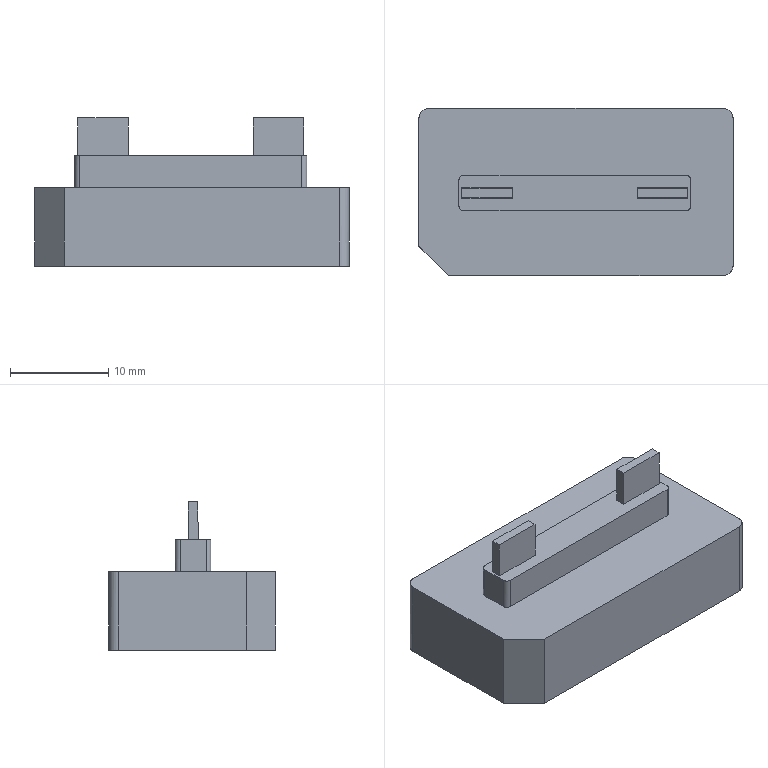NC program | PowerMill | posted by the shop | part box 32 x 17 x 15.109 mm
Lines 1 to 1617 of 35413:
%
G40 G49 G17 G80
( TOOL ID   D10C_1_1 )
( TOOL DIA. 10. TIP RAD 0 LENGTH 70.56 )
( Z = -.151 )
T1 M6
T3
G91 G28 Z0
G0 G90 G54
M08
S8000 M3
G0 X0 Y0 M8
G43 Z10.2 H1
X23.7 Y11.2
Z1.049
G1 Z-.151 F6000
X18.7 F10000
X-18.7
Y5.6
X18.7
Y0
X-18.7
Y-5.6
X18.7
Y-11.2
X-18.7
X-23.7
G0 Z10.2
X-.12 Y0
Z9.799
X24.657 Y5.134
Z.617
G1 Z-.583 F6000
X24.129 F10000
G3 X19.382 Y.387 I0 J-4.748
G1 Y-10.2
G2 X18.382 Y-11.2 I-1. J0
G1 X-18.622
G2 X-19.622 Y-10.2 I0 J1.
G1 Y10.2
G2 X-18.622 Y11.2 I1. J0
G1 X18.382
G2 X19.382 Y10.2 I0 J-1.
G1 Y.387
X16.583
Y-.387
X16.552 Y-1.16
X16.402 Y-1.934
X16.122 Y-2.736
X15.709 Y-3.48
X15.349 Y-3.96
X15.079 Y-4.254
X14.575 Y-4.701
X14.103 Y-5.027
X13.802 Y-5.199
X13.028 Y-5.529
X12.255 Y-5.723
X11.481 Y-5.792
X6.067 Y-5.793
X5.294 Y-5.706
X4.521 Y-5.499
X3.747 Y-5.153
X3.531 Y-5.027
X2.974 Y-4.632
X2.557 Y-4.254
X2.2 Y-3.855
X1.926 Y-3.48
X1.503 Y-2.707
X1.229 Y-1.934
X1.085 Y-1.16
X1.053 Y-.387
Y.387
X-1.293
Y-.387
X-1.324 Y-1.16
X-1.47 Y-1.934
X-1.667 Y-2.532
X-2.166 Y-3.48
X-2.44 Y-3.855
X-2.797 Y-4.254
X-3.214 Y-4.632
X-3.771 Y-5.027
X-3.987 Y-5.153
X-4.761 Y-5.499
X-5.534 Y-5.706
X-6.307 Y-5.793
X-11.721 Y-5.792
X-12.495 Y-5.723
X-13.268 Y-5.529
X-14.042 Y-5.199
X-14.345 Y-5.027
X-14.815 Y-4.701
X-15.319 Y-4.254
X-15.589 Y-3.96
X-15.948 Y-3.48
X-16.362 Y-2.736
X-16.648 Y-1.934
X-16.792 Y-1.16
X-16.823 Y-.387
Y.387
X-16.763 Y1.16
X-16.582 Y1.934
X-16.267 Y2.707
X-15.791 Y3.48
X-15.589 Y3.736
X-15.083 Y4.254
X-14.815 Y4.477
X-14.042 Y4.975
X-13.268 Y5.305
X-12.495 Y5.496
X-11.721 Y5.571
X-6.307 Y5.566
X-5.534 Y5.48
X-4.761 Y5.275
X-3.987 Y4.927
X-3.214 Y4.408
X-3.033 Y4.254
X-2.44 Y3.629
X-2.324 Y3.48
X-1.847 Y2.707
X-1.667 Y2.308
X-1.533 Y1.934
X-1.355 Y1.16
X-1.293 Y.387
X1.053
X1.115 Y1.16
X1.293 Y1.934
X1.427 Y2.308
X1.607 Y2.707
X2.084 Y3.48
X2.793 Y4.254
X2.974 Y4.408
X3.747 Y4.927
X4.521 Y5.275
X5.294 Y5.48
X6.067 Y5.566
X11.481 Y5.571
X12.255 Y5.496
X13.028 Y5.305
X13.7 Y5.027
X14.575 Y4.477
X14.84 Y4.254
X15.349 Y3.736
X15.552 Y3.48
X16.029 Y2.707
X16.342 Y1.934
X16.522 Y1.16
X16.583 Y.387
X19.382
G0 Z3.235
G1 X24.657 Y5.134
G0 Z.235
G1 Z-.965 F6000
X24.129 F10000
G3 X19.382 Y.387 I0 J-4.748
G1 Y-10.2
G2 X18.382 Y-11.2 I-1. J0
G1 X-18.622
G2 X-19.622 Y-10.2 I0 J1.
G1 Y10.2
G2 X-18.622 Y11.2 I1. J0
G1 X18.382
G2 X19.382 Y10.2 I0 J-1.
G1 Y.387
X16.583
Y-.387
X16.552 Y-1.16
X16.409 Y-1.934
X16.137 Y-2.707
X16.124 Y-2.73
X16.122 Y-2.736
X15.989 Y-2.977
X15.712 Y-3.48
X15.349 Y-3.963
X15.083 Y-4.254
X14.575 Y-4.705
X14.11 Y-5.027
X13.802 Y-5.203
X13.028 Y-5.533
X12.255 Y-5.726
X11.481 Y-5.798
X6.067 Y-5.797
X5.294 Y-5.712
X4.521 Y-5.504
X3.747 Y-5.158
X3.522 Y-5.027
X2.974 Y-4.638
X2.55 Y-4.254
X2.2 Y-3.862
X1.921 Y-3.48
X1.496 Y-2.707
X1.224 Y-1.934
X1.08 Y-1.16
X1.05 Y-.387
Y.387
X-1.29
Y-.387
X-1.32 Y-1.16
X-1.464 Y-1.934
X-1.667 Y-2.544
X-2.161 Y-3.48
X-2.44 Y-3.862
X-2.79 Y-4.254
X-3.214 Y-4.638
X-3.762 Y-5.027
X-3.987 Y-5.158
X-4.761 Y-5.504
X-5.534 Y-5.712
X-6.307 Y-5.797
X-11.721 Y-5.798
X-12.495 Y-5.726
X-13.268 Y-5.533
X-14.042 Y-5.203
X-14.35 Y-5.027
X-14.815 Y-4.705
X-15.323 Y-4.254
X-15.589 Y-3.963
X-15.952 Y-3.48
X-16.362 Y-2.74
X-16.649 Y-1.934
X-16.792 Y-1.16
X-16.823 Y-.387
Y.387
X-16.763 Y1.16
X-16.584 Y1.934
X-16.271 Y2.707
X-15.794 Y3.48
X-15.589 Y3.739
X-15.087 Y4.254
X-14.815 Y4.481
X-14.042 Y4.979
X-13.268 Y5.309
X-12.495 Y5.502
X-11.721 Y5.575
X-6.307 Y5.573
X-5.534 Y5.487
X-4.761 Y5.28
X-3.987 Y4.934
X-3.214 Y4.414
X-3.025 Y4.254
X-2.44 Y3.638
X-2.318 Y3.48
X-1.842 Y2.707
X-1.667 Y2.32
X-1.529 Y1.934
X-1.349 Y1.16
X-1.29 Y.387
X1.05
X1.109 Y1.16
X1.289 Y1.934
X1.427 Y2.32
X1.602 Y2.707
X2.078 Y3.48
X2.2 Y3.638
X2.785 Y4.254
X2.974 Y4.414
X3.747 Y4.934
X4.521 Y5.28
X5.294 Y5.487
X6.067 Y5.573
X11.481 Y5.575
X12.255 Y5.502
X13.028 Y5.309
X13.708 Y5.027
X14.575 Y4.481
X14.846 Y4.254
X15.349 Y3.739
X15.554 Y3.48
X16.031 Y2.707
X16.344 Y1.934
X16.523 Y1.16
X16.583 Y.387
X19.382
G0 Z2.854
G1 X24.657 Y5.134
G0 Z-.146
G1 Z-1.346 F6000
X24.129 F10000
G3 X19.382 Y.387 I0 J-4.748
G1 Y.333
X16.583 Y.387
X16.582 Y.383
Y-.387
X16.553 Y-1.139
Y-1.16
X16.41 Y-1.934
X16.138 Y-2.707
X15.714 Y-3.48
X15.349 Y-3.967
X15.086 Y-4.254
X14.575 Y-4.708
X14.116 Y-5.027
X13.802 Y-5.207
X13.028 Y-5.536
X12.255 Y-5.73
X11.552 Y-5.801
X6.078
X5.294 Y-5.715
X4.521 Y-5.509
X3.747 Y-5.163
X3.514 Y-5.027
X2.974 Y-4.644
X2.543 Y-4.254
X2.2 Y-3.87
X1.915 Y-3.48
X1.491 Y-2.707
X1.22 Y-1.934
X1.076 Y-1.16
X1.073 Y-.971
X1.05 Y-.387
Y.211
X1.047 Y.342
X-1.287 Y.387
X-1.29 Y.211
Y-.387
X-1.313 Y-.971
X-1.316 Y-1.16
X-1.46 Y-1.934
X-1.667 Y-2.555
X-2.155 Y-3.48
X-2.44 Y-3.87
X-2.783 Y-4.254
X-3.214 Y-4.644
X-3.754 Y-5.027
X-3.987 Y-5.163
X-4.761 Y-5.509
X-5.534 Y-5.715
X-6.317 Y-5.801
X-11.791
X-12.495 Y-5.73
X-13.268 Y-5.536
X-14.042 Y-5.207
X-14.356 Y-5.027
X-14.815 Y-4.708
X-15.326 Y-4.254
X-15.589 Y-3.967
X-15.954 Y-3.48
X-16.362 Y-2.743
X-16.65 Y-1.934
X-16.793 Y-1.16
Y-1.139
X-16.823 Y-.387
Y.384
Y.387
X-16.764 Y1.16
X-16.585 Y1.934
X-16.273 Y2.707
X-15.797 Y3.48
X-15.589 Y3.743
X-15.091 Y4.254
X-14.815 Y4.484
X-14.042 Y4.982
X-13.268 Y5.312
X-12.495 Y5.506
X-11.721 Y5.578
X-6.307 Y5.576
X-5.534 Y5.491
X-4.761 Y5.285
X-3.987 Y4.939
X-3.214 Y4.42
X-3.018 Y4.254
X-2.44 Y3.645
X-2.312 Y3.48
X-1.837 Y2.707
X-1.667 Y2.331
X-1.524 Y1.934
X-1.346 Y1.16
X-1.287 Y.387
X1.047 Y.342
Y.387
X1.106 Y1.16
X1.284 Y1.934
X1.427 Y2.331
X1.597 Y2.707
X2.072 Y3.48
X2.2 Y3.645
X2.778 Y4.254
X2.974 Y4.42
X3.747 Y4.939
X4.521 Y5.285
X5.294 Y5.491
X6.067 Y5.576
X11.481 Y5.578
X12.255 Y5.506
X13.028 Y5.312
X13.714 Y5.027
X14.575 Y4.484
X14.851 Y4.254
X15.349 Y3.743
X15.557 Y3.48
X16.033 Y2.707
X16.345 Y1.934
X16.524 Y1.16
X16.583 Y.387
X19.382 Y.333
Y-10.2
G2 X18.382 Y-11.2 I-1. J0
G1 X-18.622
G2 X-19.622 Y-10.2 I0 J1.
G1 Y10.2
G2 X-18.622 Y11.2 I1. J0
G1 X18.382
G2 X19.382 Y10.2 I0 J-1.
G1 Y.387
G0 Z2.472
G1 X24.657 Y5.134
G0 Z-.528
G1 Z-1.728 F6000
X24.129 F10000
G3 X19.382 Y.387 I0 J-4.748
G1 Y.333
X16.583 Y.387
X16.582 Y.38
Y-.387
X16.554 Y-1.119
X16.553 Y-1.16
X16.41 Y-1.934
X16.14 Y-2.707
X15.716 Y-3.48
X15.349 Y-3.97
X15.089 Y-4.254
X14.575 Y-4.711
X14.121 Y-5.027
X13.802 Y-5.21
X13.028 Y-5.54
X12.255 Y-5.733
X11.634 Y-5.801
X6.067 Y-5.804
X5.294 Y-5.719
X4.521 Y-5.513
X3.747 Y-5.169
X3.505 Y-5.027
X2.974 Y-4.65
X2.537 Y-4.254
X2.2 Y-3.877
X1.909 Y-3.48
X1.486 Y-2.707
X1.215 Y-1.934
X1.073 Y-1.16
X1.066 Y-.786
X1.05 Y-.387
Y.032
X1.044 Y.342
X-1.283 Y.387
X-1.29 Y.032
Y-.387
X-1.306 Y-.786
X-1.313 Y-1.16
X-1.455 Y-1.934
X-1.667 Y-2.566
X-2.149 Y-3.48
X-2.44 Y-3.877
X-2.777 Y-4.254
X-3.214 Y-4.65
X-3.745 Y-5.027
X-3.987 Y-5.169
X-4.761 Y-5.513
X-5.534 Y-5.719
X-6.232 Y-5.801
X-11.721 Y-5.806
X-11.777 Y-5.801
X-11.791
X-11.992 Y-5.78
X-12.495 Y-5.733
X-13.268 Y-5.54
X-14.042 Y-5.21
X-14.361 Y-5.027
X-14.815 Y-4.711
X-15.329 Y-4.254
X-15.589 Y-3.97
X-15.956 Y-3.48
X-16.362 Y-2.747
X-16.65 Y-1.934
X-16.793 Y-1.16
X-16.794 Y-1.119
X-16.822 Y-.387
Y.381
X-16.823 Y.387
X-16.764 Y1.16
X-16.586 Y1.934
X-16.274 Y2.707
X-15.799 Y3.48
X-15.589 Y3.746
X-15.094 Y4.254
X-14.815 Y4.487
X-14.042 Y4.986
X-13.268 Y5.315
X-12.495 Y5.509
X-11.721 Y5.582
X-6.307 Y5.58
X-5.534 Y5.495
X-4.761 Y5.289
X-3.987 Y4.944
X-3.214 Y4.426
X-3.011 Y4.254
X-2.44 Y3.653
X-2.307 Y3.48
X-1.832 Y2.707
X-1.667 Y2.342
X-1.52 Y1.934
X-1.342 Y1.16
X-1.283 Y.387
X1.044 Y.342
X1.043 Y.387
X1.102 Y1.16
X1.28 Y1.934
X1.427 Y2.342
X1.592 Y2.707
X2.067 Y3.48
X2.2 Y3.653
X2.771 Y4.254
X2.974 Y4.426
X3.747 Y4.944
X4.521 Y5.289
X5.294 Y5.495
X6.067 Y5.58
X11.481 Y5.582
X12.255 Y5.509
X13.028 Y5.315
X13.721 Y5.027
X14.575 Y4.487
X14.854 Y4.254
X15.349 Y3.746
X15.559 Y3.48
X16.034 Y2.707
X16.346 Y1.934
X16.524 Y1.16
X16.583 Y.387
X19.382 Y.333
Y-10.2
G2 X18.382 Y-11.2 I-1. J0
G1 X-18.622
G2 X-19.622 Y-10.2 I0 J1.
G1 Y10.2
G2 X-18.622 Y11.2 I1. J0
G1 X18.382
G2 X19.382 Y10.2 I0 J-1.
G1 Y.387
G0 Z2.09
G1 X24.657 Y5.134
G0 Z-.91
G1 Z-2.11 F6000
X24.129 F10000
G3 X19.382 Y.387 I0 J-4.748
G1 Y.334
X16.583 Y.387
X16.582 Y.377
Y-.387
X16.555 Y-1.1
X16.553 Y-1.16
X16.411 Y-1.934
X16.141 Y-2.707
X15.719 Y-3.48
X15.349 Y-3.973
X15.092 Y-4.254
X14.575 Y-4.715
X14.126 Y-5.027
X13.802 Y-5.213
X13.028 Y-5.543
X12.255 Y-5.736
X11.695 Y-5.801
X6.067 Y-5.807
X5.294 Y-5.723
X4.521 Y-5.518
X3.747 Y-5.174
X3.496 Y-5.027
X2.974 Y-4.656
X2.53 Y-4.254
X2.2 Y-3.884
X1.904 Y-3.48
X1.481 Y-2.707
X1.211 Y-1.934
X1.069 Y-1.16
X1.059 Y-.606
X1.05 Y-.387
Y-.151
X1.041 Y.343
X-1.28 Y.387
X-1.29 Y-.151
Y-.387
X-1.299 Y-.606
X-1.309 Y-1.16
X-1.451 Y-1.934
X-1.667 Y-2.578
X-2.144 Y-3.48
X-2.44 Y-3.884
X-2.77 Y-4.254
X-3.214 Y-4.656
X-3.736 Y-5.027
X-3.987 Y-5.174
X-4.761 Y-5.518
X-5.534 Y-5.723
X-6.168 Y-5.801
X-11.721 Y-5.809
X-12.495 Y-5.736
X-13.268 Y-5.543
X-14.042 Y-5.213
X-14.366 Y-5.027
X-14.815 Y-4.715
X-15.332 Y-4.254
X-15.589 Y-3.973
X-15.959 Y-3.48
X-16.362 Y-2.75
X-16.651 Y-1.934
X-16.793 Y-1.16
X-16.795 Y-1.1
X-16.822 Y-.387
Y.377
X-16.823 Y.387
X-16.765 Y1.16
X-16.587 Y1.934
X-16.276 Y2.707
X-15.802 Y3.48
X-15.589 Y3.749
X-15.098 Y4.254
X-14.815 Y4.491
X-14.042 Y4.989
X-13.268 Y5.319
X-12.495 Y5.512
X-11.721 Y5.585
X-6.307 Y5.583
X-5.534 Y5.499
X-4.761 Y5.294
X-3.987 Y4.95
X-3.214 Y4.432
X-3.004 Y4.254
X-2.44 Y3.66
X-2.301 Y3.48
X-1.827 Y2.707
X-1.667 Y2.354
X-1.516 Y1.934
X-1.338 Y1.16
X-1.28 Y.387
X1.041 Y.343
X1.04 Y.387
X1.098 Y1.16
X1.276 Y1.934
X1.427 Y2.354
X1.587 Y2.707
X2.061 Y3.48
X2.2 Y3.66
X2.764 Y4.254
X2.974 Y4.432
X3.747 Y4.95
X4.521 Y5.294
X5.294 Y5.499
X6.067 Y5.583
X11.481 Y5.585
X12.255 Y5.512
X13.028 Y5.319
X13.727 Y5.027
X14.575 Y4.491
X14.858 Y4.254
X15.349 Y3.749
X15.562 Y3.48
X16.036 Y2.707
X16.347 Y1.934
X16.525 Y1.16
X16.583 Y.387
X19.382 Y.334
Y-10.2
G2 X18.382 Y-11.2 I-1. J0
G1 X-18.622
G2 X-19.622 Y-10.2 I0 J1.
G1 Y10.2
G2 X-18.622 Y11.2 I1. J0
G1 X18.382
G2 X19.382 Y10.2 I0 J-1.
G1 Y.387
G0 Z1.708
G1 X24.657 Y5.134
G0 Z-1.292
G1 Z-2.492 F6000
X24.129 F10000
G3 X19.382 Y.387 I0 J-4.748
G1 Y.335
X16.583 Y.387
X16.582 Y.373
Y-.387
X16.555 Y-1.08
X16.554 Y-1.16
X16.412 Y-1.934
X16.143 Y-2.707
X15.721 Y-3.48
X15.349 Y-3.977
X15.096 Y-4.254
X14.575 Y-4.718
X14.132 Y-5.027
X13.802 Y-5.217
X13.028 Y-5.546
X12.255 Y-5.74
X11.747 Y-5.801
X6.067 Y-5.811
X5.294 Y-5.727
X4.521 Y-5.522
X3.747 Y-5.179
X3.488 Y-5.027
X2.974 Y-4.662
X2.523 Y-4.254
X2.2 Y-3.892
X1.898 Y-3.48
X1.477 Y-2.707
X1.207 Y-1.934
X1.065 Y-1.16
X1.052 Y-.43
X1.05 Y-.387
Y-.339
X1.037 Y.344
X-1.277 Y.387
X-1.29 Y-.339
Y-.387
X-1.292 Y-.43
X-1.305 Y-1.16
X-1.447 Y-1.934
X-1.667 Y-2.589
X-2.138 Y-3.48
X-2.44 Y-3.892
X-2.763 Y-4.254
X-3.214 Y-4.662
X-3.728 Y-5.027
X-3.987 Y-5.179
X-4.761 Y-5.522
X-5.534 Y-5.727
X-6.113 Y-5.801
X-11.721 Y-5.813
X-12.495 Y-5.74
X-13.268 Y-5.546
X-14.042 Y-5.217
X-14.372 Y-5.027
X-14.815 Y-4.718
X-15.336 Y-4.254
X-15.589 Y-3.977
X-15.961 Y-3.48
X-16.362 Y-2.753
X-16.652 Y-1.934
X-16.794 Y-1.16
X-16.795 Y-1.081
X-16.822 Y-.387
Y.374
X-16.823 Y.387
X-16.765 Y1.16
X-16.588 Y1.934
X-16.278 Y2.707
X-15.804 Y3.48
X-15.589 Y3.753
X-15.102 Y4.254
X-14.815 Y4.494
X-14.042 Y4.992
X-13.268 Y5.322
X-12.495 Y5.516
X-11.721 Y5.588
X-6.307 Y5.587
X-5.534 Y5.503
X-4.761 Y5.298
X-4.125 Y5.027
X-4.044 Y4.975
X-3.987 Y4.949
X-3.481 Y4.611
X-3.214 Y4.438
X-2.997 Y4.254
X-2.44 Y3.668
X-2.295 Y3.48
X-1.822 Y2.707
X-1.667 Y2.365
X-1.511 Y1.934
X-1.334 Y1.16
X-1.277 Y.387
X1.037 Y.344
Y.387
X1.094 Y1.16
X1.271 Y1.934
X1.427 Y2.365
X1.582 Y2.707
X2.055 Y3.48
X2.2 Y3.668
X2.757 Y4.254
X2.974 Y4.438
X3.747 Y4.955
X4.521 Y5.298
X5.294 Y5.503
X6.067 Y5.587
X11.481 Y5.588
X12.255 Y5.516
X13.028 Y5.322
X13.734 Y5.027
X14.575 Y4.494
X14.862 Y4.254
X15.349 Y3.753
X15.564 Y3.48
X16.038 Y2.707
X16.348 Y1.934
X16.525 Y1.16
X16.583 Y.387
X19.382 Y.335
Y-10.2
G2 X18.382 Y-11.2 I-1. J0
G1 X-18.622
G2 X-19.622 Y-10.2 I0 J1.
G1 Y10.2
G2 X-18.622 Y11.2 I1. J0
G1 X18.382
G2 X19.382 Y10.2 I0 J-1.
G1 Y.387
G0 Z1.327
G1 X24.657 Y5.134
G0 Z-1.673
G1 Z-2.873 F6000
X24.129 F10000
G3 X19.382 Y.387 I0 J-4.748
G1 Y.335
X16.583 Y.387
X16.582 Y.369
Y-.387
X16.556 Y-1.062
X16.554 Y-1.16
X16.413 Y-1.934
X16.144 Y-2.707
X15.723 Y-3.48
X15.349 Y-3.98
X15.099 Y-4.254
X14.575 Y-4.721
X14.137 Y-5.027
X13.802 Y-5.22
X13.028 Y-5.55
X12.255 Y-5.743
X11.791 Y-5.801
X6.067 Y-5.814
X5.294 Y-5.731
X4.521 Y-5.527
X3.747 Y-5.184
X3.479 Y-5.027
X2.974 Y-4.668
X2.517 Y-4.254
X2.2 Y-3.899
X1.893 Y-3.48
X1.472 Y-2.707
X1.203 Y-1.934
X1.062 Y-1.16
X1.034 Y.344
X-1.273 Y.387
X-1.302 Y-1.16
X-1.443 Y-1.934
X-1.667 Y-2.601
X-2.133 Y-3.48
X-2.44 Y-3.899
X-2.757 Y-4.254
X-3.214 Y-4.668
X-3.719 Y-5.027
X-3.987 Y-5.184
X-4.761 Y-5.527
X-5.534 Y-5.731
X-6.065 Y-5.801
X-11.721 Y-5.816
X-12.495 Y-5.743
X-13.268 Y-5.55
X-14.042 Y-5.22
X-14.377 Y-5.027
X-14.815 Y-4.721
X-15.339 Y-4.254
X-15.589 Y-3.98
X-15.963 Y-3.48
X-16.362 Y-2.757
X-16.653 Y-1.934
X-16.794 Y-1.16
X-16.796 Y-1.062
X-16.822 Y-.387
Y.371
X-16.823 Y.387
X-16.766 Y1.16
X-16.589 Y1.934
X-16.279 Y2.707
X-15.807 Y3.48
X-15.589 Y3.756
X-15.106 Y4.254
X-14.815 Y4.497
X-14.042 Y4.996
X-13.268 Y5.325
X-12.495 Y5.519
X-11.721 Y5.592
X-6.307 Y5.59
X-5.534 Y5.507
X-4.761 Y5.303
X-4.115 Y5.027
X-4.012 Y4.961
X-3.987 Y4.949
X-3.758 Y4.796
X-3.214 Y4.444
X-2.99 Y4.254
X-2.44 Y3.675
X-2.289 Y3.48
X-1.817 Y2.707
X-1.667 Y2.377
X-1.507 Y1.934
X-1.33 Y1.16
X-1.273 Y.387
X1.034 Y.344
X1.033 Y.387
X1.09 Y1.16
X1.267 Y1.934
X1.427 Y2.377
X1.577 Y2.707
X2.049 Y3.48
X2.2 Y3.675
X2.75 Y4.254
X2.974 Y4.444
X3.747 Y4.96
X4.521 Y5.303
X5.294 Y5.507
X6.067 Y5.59
X11.481 Y5.592
X12.255 Y5.519
X13.028 Y5.325
X13.741 Y5.027
X14.575 Y4.497
X14.866 Y4.254
X15.349 Y3.756
X15.567 Y3.48
X16.039 Y2.707
X16.349 Y1.934
X16.526 Y1.16
X16.583 Y.387
X19.382 Y.335
Y-10.2
G2 X18.382 Y-11.2 I-1. J0
G1 X-18.622
G2 X-19.622 Y-10.2 I0 J1.
G1 Y10.2
G2 X-18.622 Y11.2 I1. J0
G1 X18.382
G2 X19.382 Y10.2 I0 J-1.
G1 Y.387
G0 Z.945
G1 X24.657 Y5.134
G0 Z-2.055
G1 Z-3.255 F6000
X24.129 F10000
G3 X19.382 Y.387 I0 J-4.748
G1 Y.366
X16.582
Y-.387
X16.557 Y-1.044
X16.554 Y-1.16
X16.414 Y-1.934
X16.145 Y-2.707
X15.725 Y-3.48
X15.349 Y-3.983
X15.102 Y-4.254
X14.575 Y-4.725
X14.142 Y-5.027
X13.802 Y-5.223
X13.028 Y-5.553
X12.255 Y-5.746
X11.831 Y-5.801
X11.481 Y-5.819
X6.067 Y-5.818
X5.294 Y-5.735
X4.521 Y-5.531
X3.747 Y-5.189
X3.47 Y-5.027
X2.974 Y-4.674
X2.51 Y-4.254
X2.2 Y-3.907
X1.887 Y-3.48
X1.467 Y-2.707
X1.199 Y-1.934
X1.058 Y-1.16
X1.031 Y.345
X-1.27 Y.387
X-1.298 Y-1.16
X-1.439 Y-1.934
X-1.667 Y-2.612
X-2.127 Y-3.48
X-2.44 Y-3.907
X-2.75 Y-4.254
X-3.214 Y-4.674
X-3.71 Y-5.027
X-3.987 Y-5.189
X-4.761 Y-5.531
X-5.534 Y-5.735
X-6.022 Y-5.801
X-6.307 Y-5.818
X-11.721 Y-5.819
X-12.495 Y-5.746
X-13.268 Y-5.553
X-14.042 Y-5.223
X-14.382 Y-5.027
X-14.815 Y-4.725
X-15.342 Y-4.254
X-15.589 Y-3.983
X-15.965 Y-3.48
X-16.362 Y-2.76
X-16.654 Y-1.934
X-16.794 Y-1.16
X-16.797 Y-1.044
X-16.822 Y-.387
Y.368
X-16.823 Y.387
X-16.766 Y1.16
X-16.59 Y1.934
X-16.281 Y2.707
X-15.809 Y3.48
X-15.589 Y3.759
X-15.109 Y4.254
X-14.815 Y4.501
X-14.042 Y4.999
X-13.268 Y5.329
X-12.495 Y5.522
X-11.721 Y5.595
X-6.307 Y5.593
X-5.534 Y5.511
X-4.761 Y5.307
X-4.106 Y5.027
X-3.214 Y4.45
X-2.983 Y4.254
X-2.44 Y3.683
X-2.284 Y3.48
X-1.812 Y2.707
X-1.667 Y2.388
X-1.502 Y1.934
X-1.326 Y1.16
X-1.27 Y.387
X1.031 Y.345
X1.03 Y.387
X1.086 Y1.16
X1.262 Y1.934
X1.427 Y2.388
X1.572 Y2.707
X2.044 Y3.48
X2.2 Y3.683
X2.743 Y4.254
X2.974 Y4.45
X3.747 Y4.965
X4.521 Y5.307
X5.294 Y5.511
X6.067 Y5.593
X11.481 Y5.595
X12.255 Y5.522
X13.028 Y5.329
X13.747 Y5.027
X14.575 Y4.501
X14.869 Y4.254
X15.349 Y3.759
X15.569 Y3.48
X16.041 Y2.707
X16.35 Y1.934
X16.526 Y1.16
X16.583 Y.387
X16.582 Y.366
X19.382
Y-10.2
G2 X18.382 Y-11.2 I-1. J0
G1 X-18.622
G2 X-19.622 Y-10.2 I0 J1.
G1 Y10.2
G2 X-18.622 Y11.2 I1. J0
G1 X18.382
G2 X19.382 Y10.2 I0 J-1.
G1 Y.387
G0 Z.563
G1 X24.657 Y5.134
G0 Z-2.437
G1 Z-3.637 F6000
X24.129 F10000
G3 X19.382 Y.387 I0 J-4.748
G1 Y-10.2
G2 X18.382 Y-11.2 I-1. J0
G1 X-18.622
G2 X-19.622 Y-10.2 I0 J1.
G1 Y10.2
G2 X-18.622 Y11.2 I1. J0
G1 X18.382
G2 X19.382 Y10.2 I0 J-1.
G1 Y.881
X16.562 Y.677
X16.583 Y.387
X16.582 Y.362
Y-.387
X16.557 Y-1.026
X16.555 Y-1.16
X16.415 Y-1.934
X16.147 Y-2.707
X15.727 Y-3.48
X15.349 Y-3.987
X15.106 Y-4.254
X14.575 Y-4.728
X14.148 Y-5.027
X13.802 Y-5.227
X13.028 Y-5.556
X12.255 Y-5.75
X11.869 Y-5.801
X11.481 Y-5.823
X6.067 Y-5.821
X5.294 Y-5.739
X4.521 Y-5.536
X3.747 Y-5.194
X3.461 Y-5.027
X2.974 Y-4.68
X2.504 Y-4.254
X2.2 Y-3.914
X1.882 Y-3.48
X1.462 Y-2.707
X1.194 Y-1.934
X1.054 Y-1.16
X1.027 Y.346
X-1.267 Y.387
X-1.294 Y-1.16
X-1.434 Y-1.934
X-1.667 Y-2.624
X-2.122 Y-3.48
X-2.44 Y-3.914
X-2.744 Y-4.254
X-3.214 Y-4.68
X-3.701 Y-5.027
X-3.987 Y-5.194
X-4.761 Y-5.536
X-5.534 Y-5.739
X-5.981 Y-5.801
X-6.307 Y-5.821
X-11.721 Y-5.823
X-12.495 Y-5.75
X-13.268 Y-5.556
X-14.042 Y-5.227
X-14.388 Y-5.027
X-14.815 Y-4.728
X-15.346 Y-4.254
X-15.589 Y-3.987
X-15.967 Y-3.48
X-16.362 Y-2.763
X-16.655 Y-1.934
X-16.795 Y-1.16
X-16.797 Y-1.026
X-16.822 Y-.387
Y.364
X-16.823 Y.387
X-16.767 Y1.16
X-16.591 Y1.934
X-16.282 Y2.707
X-15.811 Y3.48
X-15.589 Y3.763
X-15.113 Y4.254
X-14.815 Y4.504
X-14.042 Y5.002
X-13.268 Y5.332
X-12.495 Y5.526
X-11.721 Y5.598
X-6.307 Y5.597
X-5.534 Y5.515
X-4.761 Y5.311
X-4.096 Y5.027
X-3.214 Y4.456
X-2.976 Y4.254
X-2.44 Y3.69
X-2.278 Y3.48
X-1.807 Y2.707
X-1.667 Y2.4
X-1.498 Y1.934
X-1.323 Y1.16
X-1.267 Y.387
X1.027 Y.346
Y.387
X1.083 Y1.16
X1.258 Y1.934
X1.427 Y2.4
X1.567 Y2.707
X2.038 Y3.48
X2.2 Y3.69
X2.736 Y4.254
X2.974 Y4.456
X3.747 Y4.97
X4.521 Y5.311
X5.294 Y5.515
X6.067 Y5.597
X11.481 Y5.598
X12.255 Y5.526
X13.028 Y5.332
X13.754 Y5.027
X14.575 Y4.504
X14.873 Y4.254
X15.349 Y3.763
X15.571 Y3.48
X16.042 Y2.707
X16.351 Y1.934
X16.527 Y1.16
X16.562 Y.677
X19.382 Y.881
Y.387
G0 Z.181
G1 X24.657 Y5.134
G0 Z-2.819
G1 Z-4.019 F6000
X24.129 F10000
G3 X19.382 Y.387 I0 J-4.748
G1 Y-10.2
G2 X18.382 Y-11.2 I-1. J0
G1 X-18.622
G2 X-19.622 Y-10.2 I0 J1.
G1 Y10.2
G2 X-18.622 Y11.2 I1. J0
G1 X18.382
G2 X19.382 Y10.2 I0 J-1.
G1 Y.879
X16.562 Y.677
X16.583 Y.387
X16.582 Y.358
Y-.387
X16.558 Y-1.009
X16.555 Y-1.16
X16.416 Y-1.934
X16.148 Y-2.707
X15.73 Y-3.48
X15.349 Y-3.99
X15.109 Y-4.254
X14.575 Y-4.731
X14.153 Y-5.027
X13.802 Y-5.23
X13.028 Y-5.56
X12.255 Y-5.753
X11.903 Y-5.801
X11.481 Y-5.826
X6.067 Y-5.824
X5.294 Y-5.743
X4.521 Y-5.54
X3.747 Y-5.199
X3.453 Y-5.027
X2.974 Y-4.686
X2.497 Y-4.254
X2.2 Y-3.922
X1.876 Y-3.48
X1.457 Y-2.707
X1.19 Y-1.934
X1.051 Y-1.16
X1.024 Y.346
X-1.263 Y.387
X-1.291 Y-1.16
X-1.43 Y-1.934
X-1.667 Y-2.635
X-2.116 Y-3.48
X-2.44 Y-3.922
X-2.737 Y-4.254
X-3.214 Y-4.686
X-3.693 Y-5.027
X-3.987 Y-5.199
X-4.761 Y-5.54
X-5.534 Y-5.743
X-5.943 Y-5.801
X-6.307 Y-5.824
X-11.721 Y-5.826
X-12.495 Y-5.753
X-13.268 Y-5.56
X-14.042 Y-5.23
X-14.393 Y-5.027
X-14.815 Y-4.731
X-15.349 Y-4.254
X-15.589 Y-3.99
X-15.97 Y-3.48
X-16.362 Y-2.767
X-16.656 Y-1.934
X-16.795 Y-1.16
X-16.798 Y-1.008
X-16.822 Y-.387
Y.36
X-16.823 Y.387
X-16.767 Y1.16
X-16.592 Y1.934
X-16.284 Y2.707
X-15.814 Y3.48
X-15.589 Y3.766
X-15.117 Y4.254
X-14.815 Y4.507
X-14.042 Y5.006
X-13.268 Y5.335
X-12.495 Y5.529
X-11.721 Y5.602
X-6.307 Y5.6
X-5.534 Y5.519
X-4.761 Y5.316
X-4.086 Y5.027
X-3.214 Y4.462
X-2.969 Y4.254
X-2.44 Y3.697
X-2.272 Y3.48
X-1.802 Y2.707
X-1.667 Y2.411
X-1.494 Y1.934
X-1.319 Y1.16
X-1.263 Y.387
X1.024 Y.346
X1.023 Y.387
X1.079 Y1.16
X1.254 Y1.934
X1.427 Y2.411
X1.562 Y2.707
X2.032 Y3.48
X2.2 Y3.697
X2.729 Y4.254
X2.974 Y4.462
X3.747 Y4.975
X4.521 Y5.316
X5.294 Y5.519
X6.067 Y5.6
X11.481 Y5.602
X12.255 Y5.529
X13.028 Y5.335
X13.76 Y5.027
X14.575 Y4.507
X14.877 Y4.254
X15.349 Y3.766
X15.574 Y3.48
X16.044 Y2.707
X16.352 Y1.934
X16.527 Y1.16
X16.562 Y.677
X19.382 Y.879
Y.387
G0 Z-.211
G1 X24.657 Y5.134
G0 Z-3.211
G1 Z-4.411 F6000
X24.129 F10000
G3 X19.382 Y.387 I0 J-4.748
G1 Y-10.2
G2 X18.382 Y-11.2 I-1. J0
G1 X-18.622
G2 X-19.622 Y-10.2 I0 J1.
G1 Y-1.16
X-17.123
Y1.16
X-17.071 Y1.934
X-16.92 Y2.707
X-16.648 Y3.48
X-16.236 Y4.254
X-15.648 Y5.027
X-14.815 Y5.783
X-14.042 Y6.263
X-13.329 Y6.574
X-12.495 Y6.798
X-11.721 Y6.894
X-10.948 Y6.903
X10.708
X11.481 Y6.894
X12.255 Y6.798
X13.028 Y6.596
X13.802 Y6.263
X14.551 Y5.801
X15.349 Y5.093
X15.996 Y4.254
X16.408 Y3.48
X16.68 Y2.707
X16.831 Y1.934
X16.883 Y1.16
Y-1.16
X16.858 Y-1.934
X16.736 Y-2.707
X16.5 Y-3.48
X16.129 Y-4.254
X15.6 Y-5.027
X15.349 Y-5.317
X14.835 Y-5.801
X14.575 Y-6.007
X13.63 Y-6.574
X13.028 Y-6.82
X12.255 Y-7.022
X11.481 Y-7.118
X10.708 Y-7.127
X-10.948
X-11.721 Y-7.118
X-12.495 Y-7.022
X-13.268 Y-6.82
X-13.87 Y-6.574
X-14.815 Y-6.007
X-15.075 Y-5.801
X-15.589 Y-5.317
X-15.84 Y-5.027
X-16.362 Y-4.267
X-16.74 Y-3.48
X-16.976 Y-2.707
X-17.098 Y-1.934
X-17.123 Y-1.16
X-19.622
Y10.2
G2 X-18.622 Y11.2 I1. J0
G1 X18.382
G2 X19.382 Y10.2 I0 J-1.
G1 Y.387
G0 Z-.604
G1 X24.657 Y5.134
G0 Z-3.604
G1 Z-4.804 F6000
X24.129 F10000
G3 X19.382 Y.387 I0 J-4.748
G1 Y-10.2
G2 X18.382 Y-11.2 I-1. J0
G1 X-18.622
G2 X-19.622 Y-10.2 I0 J1.
G1 Y-1.16
X-17.123
Y1.16
X-17.071 Y1.934
X-16.92 Y2.707
X-16.648 Y3.48
X-16.236 Y4.254
X-15.648 Y5.027
X-14.815 Y5.783
X-14.042 Y6.263
X-13.329 Y6.574
X-12.495 Y6.798
X-11.721 Y6.894
X-10.948 Y6.903
X10.708
X11.481 Y6.894
X12.255 Y6.798
X13.028 Y6.596
X13.802 Y6.263
X14.552 Y5.801
X15.349 Y5.093
X15.996 Y4.254
X16.408 Y3.48
X16.68 Y2.707
X16.831 Y1.934
X16.883 Y1.16
Y-1.16
X16.858 Y-1.934
X16.736 Y-2.707
X16.5 Y-3.48
X16.129 Y-4.254
X15.6 Y-5.027
X15.349 Y-5.317
X14.835 Y-5.801
X14.575 Y-6.007
X13.63 Y-6.574
X13.028 Y-6.82
X12.255 Y-7.022
X11.481 Y-7.118
X10.708 Y-7.127
X-10.948
X-11.721 Y-7.118
X-12.495 Y-7.022
X-13.268 Y-6.82
X-13.87 Y-6.574
X-14.815 Y-6.007
X-15.075 Y-5.801
X-15.589 Y-5.317
X-15.84 Y-5.027
X-16.362 Y-4.267
X-16.74 Y-3.48
X-16.976 Y-2.707
X-17.098 Y-1.934
X-17.123 Y-1.16
X-19.622
Y10.2
G2 X-18.622 Y11.2 I1. J0
G1 X18.382
G2 X19.382 Y10.2 I0 J-1.
G1 Y.387
G0 Z-.997
G1 X24.657 Y5.134
G0 Z-3.997
G1 Z-5.197 F6000
X24.129 F10000
G3 X19.382 Y.387 I0 J-4.748
G1 Y-10.2
G2 X18.382 Y-11.2 I-1. J0
G1 X-18.622
G2 X-19.622 Y-10.2 I0 J1.
G1 Y-1.16
X-17.123
Y1.16
X-17.071 Y1.934
X-16.92 Y2.707
X-16.648 Y3.48
X-16.236 Y4.254
X-15.648 Y5.027
X-14.815 Y5.783
X-14.042 Y6.263
X-13.329 Y6.574
X-12.495 Y6.798
X-11.721 Y6.894
X-10.948 Y6.903
X10.708
X11.481 Y6.894
X12.255 Y6.798
X13.028 Y6.596
X13.802 Y6.263
X14.552 Y5.801
X15.349 Y5.093
X15.996 Y4.254
X16.408 Y3.48
X16.68 Y2.707
X16.831 Y1.934
X16.883 Y1.16
Y-1.16
X16.858 Y-1.934
X16.736 Y-2.707
X16.5 Y-3.48
X16.129 Y-4.254
X15.6 Y-5.027
X15.349 Y-5.317
X14.835 Y-5.801
X14.575 Y-6.007
X13.63 Y-6.574
X13.028 Y-6.82
X12.255 Y-7.022
X11.481 Y-7.118
X10.708 Y-7.127
X-10.948
X-11.721 Y-7.118
X-12.495 Y-7.022
X-13.268 Y-6.82
X-13.87 Y-6.574
X-14.815 Y-6.007
X-15.075 Y-5.801
X-15.589 Y-5.317
X-15.84 Y-5.027
X-16.362 Y-4.267
X-16.74 Y-3.48
X-16.976 Y-2.707
X-17.098 Y-1.934
X-17.123 Y-1.16
X-19.622
Y10.2
G2 X-18.622 Y11.2 I1. J0
G1 X18.382
G2 X19.382 Y10.2 I0 J-1.
G1 Y.387
G0 Z-1.389
G1 X24.657 Y5.134
G0 Z-4.389
G1 Z-5.589 F6000
X24.129 F10000
G3 X19.382 Y.387 I0 J-4.748
G1 Y-10.2
G2 X18.382 Y-11.2 I-1. J0
G1 X-18.622
G2 X-19.622 Y-10.2 I0 J1.
G1 Y-1.16
X-17.123
Y1.16
X-17.071 Y1.934
X-16.92 Y2.707
X-16.648 Y3.48
X-16.236 Y4.254
X-15.648 Y5.027
X-14.815 Y5.783
X-14.042 Y6.263
X-13.329 Y6.574
X-12.495 Y6.798
X-11.721 Y6.894
X-10.948 Y6.903
X10.708
X11.481 Y6.894
X12.255 Y6.798
X13.028 Y6.596
X13.802 Y6.263
X14.552 Y5.801
X15.349 Y5.093
X15.996 Y4.254
X16.408 Y3.48
X16.68 Y2.707
X16.831 Y1.934
X16.883 Y1.16
Y-1.16
X16.858 Y-1.934
X16.736 Y-2.707
X16.5 Y-3.48
X16.129 Y-4.254
X15.6 Y-5.027
X15.349 Y-5.317
X14.835 Y-5.801
X14.575 Y-6.007
X13.63 Y-6.574
X13.028 Y-6.82
X12.255 Y-7.022
X11.481 Y-7.118
X10.708 Y-7.127
X-10.948
X-11.721 Y-7.118
X-12.495 Y-7.022
X-13.268 Y-6.82
X-13.87 Y-6.574
X-14.815 Y-6.007
X-15.075 Y-5.801
X-15.589 Y-5.317
X-15.84 Y-5.027
X-16.362 Y-4.267
X-16.74 Y-3.48
X-16.976 Y-2.707
X-17.098 Y-1.934
X-17.123 Y-1.16
X-19.622
Y10.2
G2 X-18.622 Y11.2 I1. J0
G1 X18.382
G2 X19.382 Y10.2 I0 J-1.
G1 Y.387
G0 Z-1.782
G1 X24.657 Y5.134
G0 Z-4.782
G1 Z-5.982 F6000
X24.129 F10000
G3 X19.382 Y.387 I0 J-4.748
G1 Y-10.2
G2 X18.382 Y-11.2 I-1. J0
G1 X-18.622
G2 X-19.622 Y-10.2 I0 J1.
G1 Y-1.16
X-17.123
Y1.16
X-17.071 Y1.934
X-16.92 Y2.707
X-16.648 Y3.48
X-16.236 Y4.254
X-15.648 Y5.027
X-14.815 Y5.783
X-14.042 Y6.263
X-13.329 Y6.574
X-12.495 Y6.798